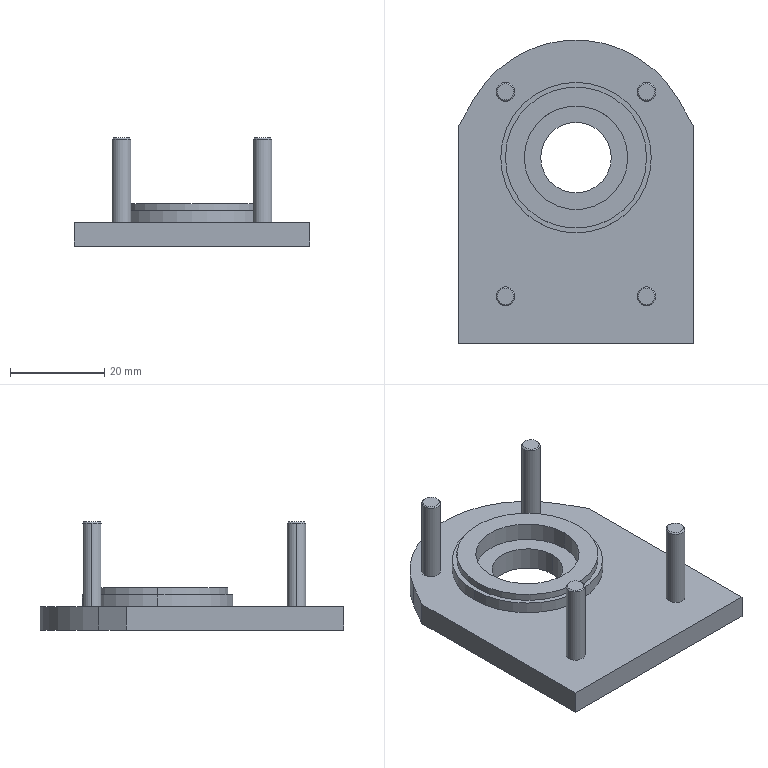Part | SolidWorks | features BaseBody 1 | 1 solid | 39 faces | box 50 x 64.5 x 23 mm | volume 16392 mm3 | cylinder 17 | plane 14 | cone 8 | commonest cylinder face diameters 4 x8 15 x2 22 x2 30 x2 32 x2 50 x1
STEP:
#1=CARTESIAN_POINT('',(-16.75,10.,23.));
#2=VERTEX_POINT('',#1);
#3=CARTESIAN_POINT('',(-13.25,10.,23.));
#4=VERTEX_POINT('',#3);
#5=CARTESIAN_POINT('',(-15.,10.,23.));
#6=DIRECTION('',(0.,0.,-1.));
#7=DIRECTION('',(-1.,0.,0.));
#8=AXIS2_PLACEMENT_3D('',#5,#6,#7);
#9=CIRCLE('',#8,1.75);
#10=EDGE_CURVE('',#2,#4,#9,.T.);
#11=ORIENTED_EDGE('',*,*,#10,.T.);
#12=CARTESIAN_POINT('',(-13.,10.,22.75));
#13=VERTEX_POINT('',#12);
#14=CARTESIAN_POINT('',(-13.125,10.,22.875));
#15=DIRECTION('',(0.7071,0.,-0.7071));
#16=VECTOR('',#15,1000.);
#17=LINE('',#14,#16);
#18=EDGE_CURVE('',#4,#13,#17,.T.);
#19=ORIENTED_EDGE('',*,*,#18,.T.);
#20=CARTESIAN_POINT('',(-17.,10.,22.75));
#21=VERTEX_POINT('',#20);
#22=CARTESIAN_POINT('',(-15.,10.,22.75));
#23=DIRECTION('',(0.,0.,1.));
#24=DIRECTION('',(-1.,0.,0.));
#25=AXIS2_PLACEMENT_3D('',#22,#23,#24);
#26=CIRCLE('',#25,2.);
#27=EDGE_CURVE('',#13,#21,#26,.T.);
#28=ORIENTED_EDGE('',*,*,#27,.T.);
#29=CARTESIAN_POINT('',(-16.875,10.,22.875));
#30=DIRECTION('',(-0.7071,0.,-0.7071));
#31=VECTOR('',#30,1000.);
#32=LINE('',#29,#31);
#33=EDGE_CURVE('',#2,#21,#32,.T.);
#34=ORIENTED_EDGE('',*,*,#33,.F.);
#35=EDGE_LOOP('',(#11,#19,#28,#34));
#36=FACE_OUTER_BOUND('',#35,.T.);
#37=CARTESIAN_POINT('',(-15.,10.,22.875));
#38=DIRECTION('',(0.,0.,-1.));
#39=DIRECTION('',(-1.,0.,0.));
#40=AXIS2_PLACEMENT_3D('',#37,#38,#39);
#41=CONICAL_SURFACE('',#40,1.875,0.7854);
#42=ADVANCED_FACE('',(#36),#41,.T.);
#43=ORIENTED_EDGE('',*,*,#27,.F.);
#44=CARTESIAN_POINT('',(-13.,10.,5.));
#45=VERTEX_POINT('',#44);
#46=CARTESIAN_POINT('',(-13.,10.,5.));
#47=DIRECTION('',(0.,0.,-1.));
#48=VECTOR('',#47,1000.);
#49=LINE('',#46,#48);
#50=EDGE_CURVE('',#13,#45,#49,.T.);
#51=ORIENTED_EDGE('',*,*,#50,.T.);
#52=CARTESIAN_POINT('',(-17.,10.,5.));
#53=VERTEX_POINT('',#52);
#54=CARTESIAN_POINT('',(-15.,10.,5.));
#55=DIRECTION('',(0.,0.,-1.));
#56=DIRECTION('',(-1.,0.,0.));
#57=AXIS2_PLACEMENT_3D('',#54,#55,#56);
#58=CIRCLE('',#57,2.);
#59=EDGE_CURVE('',#53,#45,#58,.T.);
#60=ORIENTED_EDGE('',*,*,#59,.F.);
#61=CARTESIAN_POINT('',(-17.,10.,5.));
#62=DIRECTION('',(0.,0.,-1.));
#63=VECTOR('',#62,1000.);
#64=LINE('',#61,#63);
#65=EDGE_CURVE('',#21,#53,#64,.T.);
#66=ORIENTED_EDGE('',*,*,#65,.F.);
#67=EDGE_LOOP('',(#43,#51,#60,#66));
#68=FACE_OUTER_BOUND('',#67,.T.);
#69=CARTESIAN_POINT('',(-15.,10.,5.));
#70=DIRECTION('',(0.,0.,-1.));
#71=DIRECTION('',(-1.,0.,0.));
#72=AXIS2_PLACEMENT_3D('',#69,#70,#71);
#73=CYLINDRICAL_SURFACE('',#72,2.);
#74=ADVANCED_FACE('',(#68),#73,.T.);
#75=CARTESIAN_POINT('',(13.25,10.,23.));
#76=VERTEX_POINT('',#75);
#77=CARTESIAN_POINT('',(16.75,10.,23.));
#78=VERTEX_POINT('',#77);
#79=CARTESIAN_POINT('',(15.,10.,23.));
#80=DIRECTION('',(0.,0.,-1.));
#81=DIRECTION('',(-1.,0.,0.));
#82=AXIS2_PLACEMENT_3D('',#79,#80,#81);
#83=CIRCLE('',#82,1.75);
#84=EDGE_CURVE('',#76,#78,#83,.T.);
#85=ORIENTED_EDGE('',*,*,#84,.T.);
#86=CARTESIAN_POINT('',(17.,10.,22.75));
#87=VERTEX_POINT('',#86);
#88=CARTESIAN_POINT('',(16.875,10.,22.875));
#89=DIRECTION('',(0.7071,0.,-0.7071));
#90=VECTOR('',#89,1000.);
#91=LINE('',#88,#90);
#92=EDGE_CURVE('',#78,#87,#91,.T.);
#93=ORIENTED_EDGE('',*,*,#92,.T.);
#94=CARTESIAN_POINT('',(13.,10.,22.75));
#95=VERTEX_POINT('',#94);
#96=CARTESIAN_POINT('',(15.,10.,22.75));
#97=DIRECTION('',(0.,0.,1.));
#98=DIRECTION('',(-1.,0.,0.));
#99=AXIS2_PLACEMENT_3D('',#96,#97,#98);
#100=CIRCLE('',#99,2.);
#101=EDGE_CURVE('',#87,#95,#100,.T.);
#102=ORIENTED_EDGE('',*,*,#101,.T.);
#103=CARTESIAN_POINT('',(13.125,10.,22.875));
#104=DIRECTION('',(-0.7071,0.,-0.7071));
#105=VECTOR('',#104,1000.);
#106=LINE('',#103,#105);
#107=EDGE_CURVE('',#76,#95,#106,.T.);
#108=ORIENTED_EDGE('',*,*,#107,.F.);
#109=EDGE_LOOP('',(#85,#93,#102,#108));
#110=FACE_OUTER_BOUND('',#109,.T.);
#111=CARTESIAN_POINT('',(15.,10.,22.875));
#112=DIRECTION('',(0.,0.,-1.));
#113=DIRECTION('',(-1.,0.,0.));
#114=AXIS2_PLACEMENT_3D('',#111,#112,#113);
#115=CONICAL_SURFACE('',#114,1.875,0.7854);
#116=ADVANCED_FACE('',(#110),#115,.T.);
#117=ORIENTED_EDGE('',*,*,#101,.F.);
#118=CARTESIAN_POINT('',(17.,10.,5.));
#119=VERTEX_POINT('',#118);
#120=CARTESIAN_POINT('',(17.,10.,5.));
#121=DIRECTION('',(0.,0.,-1.));
#122=VECTOR('',#121,1000.);
#123=LINE('',#120,#122);
#124=EDGE_CURVE('',#87,#119,#123,.T.);
#125=ORIENTED_EDGE('',*,*,#124,.T.);
#126=CARTESIAN_POINT('',(13.,10.,5.));
#127=VERTEX_POINT('',#126);
#128=CARTESIAN_POINT('',(15.,10.,5.));
#129=DIRECTION('',(0.,0.,-1.));
#130=DIRECTION('',(-1.,0.,0.));
#131=AXIS2_PLACEMENT_3D('',#128,#129,#130);
#132=CIRCLE('',#131,2.);
#133=EDGE_CURVE('',#127,#119,#132,.T.);
#134=ORIENTED_EDGE('',*,*,#133,.F.);
#135=CARTESIAN_POINT('',(13.,10.,5.));
#136=DIRECTION('',(0.,0.,-1.));
#137=VECTOR('',#136,1000.);
#138=LINE('',#135,#137);
#139=EDGE_CURVE('',#95,#127,#138,.T.);
#140=ORIENTED_EDGE('',*,*,#139,.F.);
#141=EDGE_LOOP('',(#117,#125,#134,#140));
#142=FACE_OUTER_BOUND('',#141,.T.);
#143=CARTESIAN_POINT('',(15.,10.,5.));
#144=DIRECTION('',(0.,0.,-1.));
#145=DIRECTION('',(-1.,0.,0.));
#146=AXIS2_PLACEMENT_3D('',#143,#144,#145);
#147=CYLINDRICAL_SURFACE('',#146,2.);
#148=ADVANCED_FACE('',(#142),#147,.T.);
#149=CARTESIAN_POINT('',(13.25,53.473,23.));
#150=VERTEX_POINT('',#149);
#151=CARTESIAN_POINT('',(16.75,53.473,23.));
#152=VERTEX_POINT('',#151);
#153=CARTESIAN_POINT('',(15.,53.473,23.));
#154=DIRECTION('',(0.,0.,-1.));
#155=DIRECTION('',(-1.,0.,0.));
#156=AXIS2_PLACEMENT_3D('',#153,#154,#155);
#157=CIRCLE('',#156,1.75);
#158=EDGE_CURVE('',#150,#152,#157,.T.);
#159=ORIENTED_EDGE('',*,*,#158,.T.);
#160=CARTESIAN_POINT('',(17.,53.473,22.75));
#161=VERTEX_POINT('',#160);
#162=CARTESIAN_POINT('',(16.875,53.473,22.875));
#163=DIRECTION('',(0.7071,0.,-0.7071));
#164=VECTOR('',#163,1000.);
#165=LINE('',#162,#164);
#166=EDGE_CURVE('',#152,#161,#165,.T.);
#167=ORIENTED_EDGE('',*,*,#166,.T.);
#168=CARTESIAN_POINT('',(13.,53.473,22.75));
#169=VERTEX_POINT('',#168);
#170=CARTESIAN_POINT('',(15.,53.473,22.75));
#171=DIRECTION('',(0.,0.,1.));
#172=DIRECTION('',(-1.,0.,0.));
#173=AXIS2_PLACEMENT_3D('',#170,#171,#172);
#174=CIRCLE('',#173,2.);
#175=EDGE_CURVE('',#161,#169,#174,.T.);
#176=ORIENTED_EDGE('',*,*,#175,.T.);
#177=CARTESIAN_POINT('',(13.125,53.473,22.875));
#178=DIRECTION('',(-0.7071,0.,-0.7071));
#179=VECTOR('',#178,1000.);
#180=LINE('',#177,#179);
#181=EDGE_CURVE('',#150,#169,#180,.T.);
#182=ORIENTED_EDGE('',*,*,#181,.F.);
#183=EDGE_LOOP('',(#159,#167,#176,#182));
#184=FACE_OUTER_BOUND('',#183,.T.);
#185=CARTESIAN_POINT('',(15.,53.473,22.875));
#186=DIRECTION('',(0.,0.,-1.));
#187=DIRECTION('',(-1.,0.,0.));
#188=AXIS2_PLACEMENT_3D('',#185,#186,#187);
#189=CONICAL_SURFACE('',#188,1.875,0.7854);
#190=ADVANCED_FACE('',(#184),#189,.T.);
#191=ORIENTED_EDGE('',*,*,#175,.F.);
#192=CARTESIAN_POINT('',(17.,53.473,5.));
#193=VERTEX_POINT('',#192);
#194=CARTESIAN_POINT('',(17.,53.473,5.));
#195=DIRECTION('',(0.,0.,-1.));
#196=VECTOR('',#195,1000.);
#197=LINE('',#194,#196);
#198=EDGE_CURVE('',#161,#193,#197,.T.);
#199=ORIENTED_EDGE('',*,*,#198,.T.);
#200=CARTESIAN_POINT('',(13.,53.473,5.));
#201=VERTEX_POINT('',#200);
#202=CARTESIAN_POINT('',(15.,53.473,5.));
#203=DIRECTION('',(0.,0.,-1.));
#204=DIRECTION('',(-1.,0.,0.));
#205=AXIS2_PLACEMENT_3D('',#202,#203,#204);
#206=CIRCLE('',#205,2.);
#207=EDGE_CURVE('',#201,#193,#206,.T.);
#208=ORIENTED_EDGE('',*,*,#207,.F.);
#209=CARTESIAN_POINT('',(13.,53.473,5.));
#210=DIRECTION('',(0.,0.,-1.));
#211=VECTOR('',#210,1000.);
#212=LINE('',#209,#211);
#213=EDGE_CURVE('',#169,#201,#212,.T.);
#214=ORIENTED_EDGE('',*,*,#213,.F.);
#215=EDGE_LOOP('',(#191,#199,#208,#214));
#216=FACE_OUTER_BOUND('',#215,.T.);
#217=CARTESIAN_POINT('',(15.,53.473,5.));
#218=DIRECTION('',(0.,0.,-1.));
#219=DIRECTION('',(-1.,0.,0.));
#220=AXIS2_PLACEMENT_3D('',#217,#218,#219);
#221=CYLINDRICAL_SURFACE('',#220,2.);
#222=ADVANCED_FACE('',(#216),#221,.T.);
#223=CARTESIAN_POINT('',(-16.75,53.473,23.));
#224=VERTEX_POINT('',#223);
#225=CARTESIAN_POINT('',(-13.25,53.473,23.));
#226=VERTEX_POINT('',#225);
#227=CARTESIAN_POINT('',(-15.,53.473,23.));
#228=DIRECTION('',(0.,0.,-1.));
#229=DIRECTION('',(-1.,0.,0.));
#230=AXIS2_PLACEMENT_3D('',#227,#228,#229);
#231=CIRCLE('',#230,1.75);
#232=EDGE_CURVE('',#224,#226,#231,.T.);
#233=ORIENTED_EDGE('',*,*,#232,.T.);
#234=CARTESIAN_POINT('',(-13.,53.473,22.75));
#235=VERTEX_POINT('',#234);
#236=CARTESIAN_POINT('',(-13.125,53.473,22.875));
#237=DIRECTION('',(0.7071,0.,-0.7071));
#238=VECTOR('',#237,1000.);
#239=LINE('',#236,#238);
#240=EDGE_CURVE('',#226,#235,#239,.T.);
#241=ORIENTED_EDGE('',*,*,#240,.T.);
#242=CARTESIAN_POINT('',(-17.,53.473,22.75));
#243=VERTEX_POINT('',#242);
#244=CARTESIAN_POINT('',(-15.,53.473,22.75));
#245=DIRECTION('',(0.,0.,1.));
#246=DIRECTION('',(-1.,0.,0.));
#247=AXIS2_PLACEMENT_3D('',#244,#245,#246);
#248=CIRCLE('',#247,2.);
#249=EDGE_CURVE('',#235,#243,#248,.T.);
#250=ORIENTED_EDGE('',*,*,#249,.T.);
#251=CARTESIAN_POINT('',(-16.875,53.473,22.875));
#252=DIRECTION('',(-0.7071,0.,-0.7071));
#253=VECTOR('',#252,1000.);
#254=LINE('',#251,#253);
#255=EDGE_CURVE('',#224,#243,#254,.T.);
#256=ORIENTED_EDGE('',*,*,#255,.F.);
#257=EDGE_LOOP('',(#233,#241,#250,#256));
#258=FACE_OUTER_BOUND('',#257,.T.);
#259=CARTESIAN_POINT('',(-15.,53.473,22.875));
#260=DIRECTION('',(0.,0.,-1.));
#261=DIRECTION('',(-1.,0.,0.));
#262=AXIS2_PLACEMENT_3D('',#259,#260,#261);
#263=CONICAL_SURFACE('',#262,1.875,0.7854);
#264=ADVANCED_FACE('',(#258),#263,.T.);
#265=ORIENTED_EDGE('',*,*,#249,.F.);
#266=CARTESIAN_POINT('',(-13.,53.473,5.));
#267=VERTEX_POINT('',#266);
#268=CARTESIAN_POINT('',(-13.,53.473,5.));
#269=DIRECTION('',(0.,0.,-1.));
#270=VECTOR('',#269,1000.);
#271=LINE('',#268,#270);
#272=EDGE_CURVE('',#235,#267,#271,.T.);
#273=ORIENTED_EDGE('',*,*,#272,.T.);
#274=CARTESIAN_POINT('',(-17.,53.473,5.));
#275=VERTEX_POINT('',#274);
#276=CARTESIAN_POINT('',(-15.,53.473,5.));
#277=DIRECTION('',(0.,0.,-1.));
#278=DIRECTION('',(-1.,0.,0.));
#279=AXIS2_PLACEMENT_3D('',#276,#277,#278);
#280=CIRCLE('',#279,2.);
#281=EDGE_CURVE('',#275,#267,#280,.T.);
#282=ORIENTED_EDGE('',*,*,#281,.F.);
#283=CARTESIAN_POINT('',(-17.,53.473,5.));
#284=DIRECTION('',(0.,0.,-1.));
#285=VECTOR('',#284,1000.);
#286=LINE('',#283,#285);
#287=EDGE_CURVE('',#243,#275,#286,.T.);
#288=ORIENTED_EDGE('',*,*,#287,.F.);
#289=EDGE_LOOP('',(#265,#273,#282,#288));
#290=FACE_OUTER_BOUND('',#289,.T.);
#291=CARTESIAN_POINT('',(-15.,53.473,5.));
#292=DIRECTION('',(0.,0.,-1.));
#293=DIRECTION('',(-1.,0.,0.));
#294=AXIS2_PLACEMENT_3D('',#291,#292,#293);
#295=CYLINDRICAL_SURFACE('',#294,2.);
#296=ADVANCED_FACE('',(#290),#295,.T.);
#297=CARTESIAN_POINT('',(7.5,39.5,0.));
#298=VERTEX_POINT('',#297);
#299=CARTESIAN_POINT('',(-7.5,39.5,0.));
#300=VERTEX_POINT('',#299);
#301=CARTESIAN_POINT('',(0.,39.5,0.));
#302=DIRECTION('',(0.,0.,1.));
#303=DIRECTION('',(-1.,0.,0.));
#304=AXIS2_PLACEMENT_3D('',#301,#302,#303);
#305=CIRCLE('',#304,7.5);
#306=EDGE_CURVE('',#298,#300,#305,.T.);
#307=ORIENTED_EDGE('',*,*,#306,.F.);
#308=CARTESIAN_POINT('',(7.5,39.5,5.));
#309=VERTEX_POINT('',#308);
#310=CARTESIAN_POINT('',(7.5,39.5,5.));
#311=DIRECTION('',(0.,0.,1.));
#312=VECTOR('',#311,1000.);
#313=LINE('',#310,#312);
#314=EDGE_CURVE('',#298,#309,#313,.T.);
#315=ORIENTED_EDGE('',*,*,#314,.T.);
#316=CARTESIAN_POINT('',(-7.5,39.5,5.));
#317=VERTEX_POINT('',#316);
#318=CARTESIAN_POINT('',(0.,39.5,5.));
#319=DIRECTION('',(0.,0.,-1.));
#320=DIRECTION('',(-1.,0.,0.));
#321=AXIS2_PLACEMENT_3D('',#318,#319,#320);
#322=CIRCLE('',#321,7.5);
#323=EDGE_CURVE('',#317,#309,#322,.T.);
#324=ORIENTED_EDGE('',*,*,#323,.F.);
#325=CARTESIAN_POINT('',(-7.5,39.5,5.));
#326=DIRECTION('',(0.,0.,1.));
#327=VECTOR('',#326,1000.);
#328=LINE('',#325,#327);
#329=EDGE_CURVE('',#300,#317,#328,.T.);
#330=ORIENTED_EDGE('',*,*,#329,.F.);
#331=EDGE_LOOP('',(#307,#315,#324,#330));
#332=FACE_OUTER_BOUND('',#331,.T.);
#333=CARTESIAN_POINT('',(0.,39.5,5.));
#334=DIRECTION('',(0.,0.,1.));
#335=DIRECTION('',(-1.,0.,0.));
#336=AXIS2_PLACEMENT_3D('',#333,#334,#335);
#337=CYLINDRICAL_SURFACE('',#336,7.5);
#338=ADVANCED_FACE('',(#332),#337,.F.);
#339=CARTESIAN_POINT('',(-15.,39.5,7.5));
#340=VERTEX_POINT('',#339);
#341=CARTESIAN_POINT('',(15.,39.5,7.5));
#342=VERTEX_POINT('',#341);
#343=CARTESIAN_POINT('',(0.,39.5,7.5));
#344=DIRECTION('',(0.,0.,1.));
#345=DIRECTION('',(-1.,0.,0.));
#346=AXIS2_PLACEMENT_3D('',#343,#344,#345);
#347=CIRCLE('',#346,15.);
#348=EDGE_CURVE('',#340,#342,#347,.T.);
#349=ORIENTED_EDGE('',*,*,#348,.T.);
#350=CARTESIAN_POINT('',(15.,39.5,9.));
#351=VERTEX_POINT('',#350);
#352=CARTESIAN_POINT('',(15.,39.5,9.));
#353=DIRECTION('',(0.,0.,1.));
#354=VECTOR('',#353,1000.);
#355=LINE('',#352,#354);
#356=EDGE_CURVE('',#342,#351,#355,.T.);
#357=ORIENTED_EDGE('',*,*,#356,.T.);
#358=CARTESIAN_POINT('',(-15.,39.5,9.));
#359=VERTEX_POINT('',#358);
#360=CARTESIAN_POINT('',(0.,39.5,9.));
#361=DIRECTION('',(0.,0.,1.));
#362=DIRECTION('',(-1.,0.,0.));
#363=AXIS2_PLACEMENT_3D('',#360,#361,#362);
#364=CIRCLE('',#363,15.);
#365=EDGE_CURVE('',#359,#351,#364,.T.);
#366=ORIENTED_EDGE('',*,*,#365,.F.);
#367=CARTESIAN_POINT('',(-15.,39.5,9.));
#368=DIRECTION('',(0.,0.,1.));
#369=VECTOR('',#368,1000.);
#370=LINE('',#367,#369);
#371=EDGE_CURVE('',#340,#359,#370,.T.);
#372=ORIENTED_EDGE('',*,*,#371,.F.);
#373=EDGE_LOOP('',(#349,#357,#366,#372));
#374=FACE_OUTER_BOUND('',#373,.T.);
#375=CARTESIAN_POINT('',(0.,39.5,9.));
#376=DIRECTION('',(0.,0.,1.));
#377=DIRECTION('',(-1.,0.,0.));
#378=AXIS2_PLACEMENT_3D('',#375,#376,#377);
#379=CYLINDRICAL_SURFACE('',#378,15.);
#380=ADVANCED_FACE('',(#374),#379,.T.);
#381=CARTESIAN_POINT('',(11.,39.5,9.));
#382=VERTEX_POINT('',#381);
#383=CARTESIAN_POINT('',(-11.,39.5,9.));
#384=VERTEX_POINT('',#383);
#385=CARTESIAN_POINT('',(0.,39.5,9.));
#386=DIRECTION('',(0.,0.,-1.));
#387=DIRECTION('',(-1.,0.,0.));
#388=AXIS2_PLACEMENT_3D('',#385,#386,#387);
#389=CIRCLE('',#388,11.);
#390=EDGE_CURVE('',#382,#384,#389,.T.);
#391=ORIENTED_EDGE('',*,*,#390,.F.);
#392=CARTESIAN_POINT('',(11.,39.5,5.));
#393=VERTEX_POINT('',#392);
#394=CARTESIAN_POINT('',(11.,39.5,5.));
#395=DIRECTION('',(0.,0.,-1.));
#396=VECTOR('',#395,1000.);
#397=LINE('',#394,#396);
#398=EDGE_CURVE('',#382,#393,#397,.T.);
#399=ORIENTED_EDGE('',*,*,#398,.T.);
#400=CARTESIAN_POINT('',(-11.,39.5,5.));
#401=VERTEX_POINT('',#400);
#402=CARTESIAN_POINT('',(0.,39.5,5.));
#403=DIRECTION('',(0.,0.,1.));
#404=DIRECTION('',(-1.,0.,0.));
#405=AXIS2_PLACEMENT_3D('',#402,#403,#404);
#406=CIRCLE('',#405,11.);
#407=EDGE_CURVE('',#401,#393,#406,.T.);
#408=ORIENTED_EDGE('',*,*,#407,.F.);
#409=CARTESIAN_POINT('',(-11.,39.5,5.));
#410=DIRECTION('',(0.,0.,-1.));
#411=VECTOR('',#410,1000.);
#412=LINE('',#409,#411);
#413=EDGE_CURVE('',#384,#401,#412,.T.);
#414=ORIENTED_EDGE('',*,*,#413,.F.);
#415=EDGE_LOOP('',(#391,#399,#408,#414));
#416=FACE_OUTER_BOUND('',#415,.T.);
#417=CARTESIAN_POINT('',(0.,39.5,5.));
#418=DIRECTION('',(0.,0.,-1.));
#419=DIRECTION('',(-1.,0.,0.));
#420=AXIS2_PLACEMENT_3D('',#417,#418,#419);
#421=CYLINDRICAL_SURFACE('',#420,11.);
#422=ADVANCED_FACE('',(#416),#421,.F.);
#423=CARTESIAN_POINT('',(-16.,39.5,7.5));
#424=VERTEX_POINT('',#423);
#425=CARTESIAN_POINT('',(16.,39.5,7.5));
#426=VERTEX_POINT('',#425);
#427=CARTESIAN_POINT('',(0.,39.5,7.5));
#428=DIRECTION('',(0.,0.,-1.));
#429=DIRECTION('',(-1.,0.,0.));
#430=AXIS2_PLACEMENT_3D('',#427,#428,#429);
#431=CIRCLE('',#430,16.);
#432=EDGE_CURVE('',#424,#426,#431,.T.);
#433=ORIENTED_EDGE('',*,*,#432,.T.);
#434=CARTESIAN_POINT('',(16.,39.5,5.));
#435=VERTEX_POINT('',#434);
#436=CARTESIAN_POINT('',(16.,39.5,5.));
#437=DIRECTION('',(0.,0.,-1.));
#438=VECTOR('',#437,1000.);
#439=LINE('',#436,#438);
#440=EDGE_CURVE('',#426,#435,#439,.T.);
#441=ORIENTED_EDGE('',*,*,#440,.T.);
#442=CARTESIAN_POINT('',(-16.,39.5,5.));
#443=VERTEX_POINT('',#442);
#444=CARTESIAN_POINT('',(0.,39.5,5.));
#445=DIRECTION('',(0.,0.,-1.));
#446=DIRECTION('',(-1.,0.,0.));
#447=AXIS2_PLACEMENT_3D('',#444,#445,#446);
#448=CIRCLE('',#447,16.);
#449=EDGE_CURVE('',#443,#435,#448,.T.);
#450=ORIENTED_EDGE('',*,*,#449,.F.);
#451=CARTESIAN_POINT('',(-16.,39.5,5.));
#452=DIRECTION('',(0.,0.,-1.));
#453=VECTOR('',#452,1000.);
#454=LINE('',#451,#453);
#455=EDGE_CURVE('',#424,#443,#454,.T.);
#456=ORIENTED_EDGE('',*,*,#455,.F.);
#457=EDGE_LOOP('',(#433,#441,#450,#456));
#458=FACE_OUTER_BOUND('',#457,.T.);
#459=CARTESIAN_POINT('',(0.,39.5,5.));
#460=DIRECTION('',(0.,0.,-1.));
#461=DIRECTION('',(-1.,0.,0.));
#462=AXIS2_PLACEMENT_3D('',#459,#460,#461);
#463=CYLINDRICAL_SURFACE('',#462,16.);
#464=ADVANCED_FACE('',(#458),#463,.T.);
#465=ORIENTED_EDGE('',*,*,#10,.F.);
#466=CARTESIAN_POINT('',(-15.,10.,23.));
#467=DIRECTION('',(0.,0.,-1.));
#468=DIRECTION('',(-1.,0.,0.));
#469=AXIS2_PLACEMENT_3D('',#466,#467,#468);
#470=CIRCLE('',#469,1.75);
#471=EDGE_CURVE('',#4,#2,#470,.T.);
#472=ORIENTED_EDGE('',*,*,#471,.F.);
#473=EDGE_LOOP('',(#465,#472));
#474=FACE_OUTER_BOUND('',#473,.T.);
#475=CARTESIAN_POINT('',(-15.,10.,23.));
#476=DIRECTION('',(0.,0.,1.));
#477=DIRECTION('',(1.,0.,0.));
#478=AXIS2_PLACEMENT_3D('',#475,#476,#477);
#479=PLANE('',#478);
#480=ADVANCED_FACE('',(#474),#479,.T.);
#481=ORIENTED_EDGE('',*,*,#84,.F.);
#482=CARTESIAN_POINT('',(15.,10.,23.));
#483=DIRECTION('',(0.,0.,-1.));
#484=DIRECTION('',(-1.,0.,0.));
#485=AXIS2_PLACEMENT_3D('',#482,#483,#484);
#486=CIRCLE('',#485,1.75);
#487=EDGE_CURVE('',#78,#76,#486,.T.);
#488=ORIENTED_EDGE('',*,*,#487,.F.);
#489=EDGE_LOOP('',(#481,#488));
#490=FACE_OUTER_BOUND('',#489,.T.);
#491=CARTESIAN_POINT('',(15.,10.,23.));
#492=DIRECTION('',(0.,0.,1.));
#493=DIRECTION('',(1.,0.,0.));
#494=AXIS2_PLACEMENT_3D('',#491,#492,#493);
#495=PLANE('',#494);
#496=ADVANCED_FACE('',(#490),#495,.T.);
#497=ORIENTED_EDGE('',*,*,#158,.F.);
#498=CARTESIAN_POINT('',(15.,53.473,23.));
#499=DIRECTION('',(0.,0.,-1.));
#500=DIRECTION('',(-1.,0.,0.));
#501=AXIS2_PLACEMENT_3D('',#498,#499,#500);
#502=CIRCLE('',#501,1.75);
#503=EDGE_CURVE('',#152,#150,#502,.T.);
#504=ORIENTED_EDGE('',*,*,#503,.F.);
#505=EDGE_LOOP('',(#497,#504));
#506=FACE_OUTER_BOUND('',#505,.T.);
#507=CARTESIAN_POINT('',(15.,53.473,23.));
#508=DIRECTION('',(0.,0.,1.));
#509=DIRECTION('',(1.,0.,0.));
#510=AXIS2_PLACEMENT_3D('',#507,#508,#509);
#511=PLANE('',#510);
#512=ADVANCED_FACE('',(#506),#511,.T.);
#513=ORIENTED_EDGE('',*,*,#232,.F.);
#514=CARTESIAN_POINT('',(-15.,53.473,23.));
#515=DIRECTION('',(0.,0.,-1.));
#516=DIRECTION('',(-1.,0.,0.));
#517=AXIS2_PLACEMENT_3D('',#514,#515,#516);
#518=CIRCLE('',#517,1.75);
#519=EDGE_CURVE('',#226,#224,#518,.T.);
#520=ORIENTED_EDGE('',*,*,#519,.F.);
#521=EDGE_LOOP('',(#513,#520));
#522=FACE_OUTER_BOUND('',#521,.T.);
#523=CARTESIAN_POINT('',(-15.,53.473,23.));
#524=DIRECTION('',(0.,0.,1.));
#525=DIRECTION('',(1.,0.,0.));
#526=AXIS2_PLACEMENT_3D('',#523,#524,#525);
#527=PLANE('',#526);
#528=ADVANCED_FACE('',(#522),#527,.T.);
#529=ORIENTED_EDGE('',*,*,#348,.F.);
#530=CARTESIAN_POINT('',(0.,39.5,7.5));
#531=DIRECTION('',(0.,0.,1.));
#532=DIRECTION('',(-1.,0.,0.));
#533=AXIS2_PLACEMENT_3D('',#530,#531,#532);
#534=CIRCLE('',#533,15.);
#535=EDGE_CURVE('',#342,#340,#534,.T.);
#536=ORIENTED_EDGE('',*,*,#535,.F.);
#537=EDGE_LOOP('',(#529,#536));
#538=FACE_BOUND('',#537,.T.);
#539=ORIENTED_EDGE('',*,*,#432,.F.);
#540=CARTESIAN_POINT('',(0.,39.5,7.5));
#541=DIRECTION('',(0.,0.,-1.));
#542=DIRECTION('',(-1.,0.,0.));
#543=AXIS2_PLACEMENT_3D('',#540,#541,#542);
#544=CIRCLE('',#543,16.);
#545=EDGE_CURVE('',#426,#424,#544,.T.);
#546=ORIENTED_EDGE('',*,*,#545,.F.);
#547=EDGE_LOOP('',(#539,#546));
#548=FACE_OUTER_BOUND('',#547,.T.);
#549=CARTESIAN_POINT('',(0.,39.5,7.5));
#550=DIRECTION('',(0.,0.,1.));
#551=DIRECTION('',(1.,0.,0.));
#552=AXIS2_PLACEMENT_3D('',#549,#550,#551);
#553=PLANE('',#552);
#554=ADVANCED_FACE('',(#538,#548),#553,.T.);
#555=CARTESIAN_POINT('',(0.,39.5,9.));
#556=DIRECTION('',(0.,0.,-1.));
#557=DIRECTION('',(-1.,0.,0.));
#558=AXIS2_PLACEMENT_3D('',#555,#556,#557);
#559=CIRCLE('',#558,11.);
#560=EDGE_CURVE('',#384,#382,#559,.T.);
#561=ORIENTED_EDGE('',*,*,#560,.T.);
#562=ORIENTED_EDGE('',*,*,#390,.T.);
#563=EDGE_LOOP('',(#561,#562));
#564=FACE_BOUND('',#563,.T.);
#565=ORIENTED_EDGE('',*,*,#365,.T.);
#566=CARTESIAN_POINT('',(0.,39.5,9.));
#567=DIRECTION('',(0.,0.,1.));
#568=DIRECTION('',(-1.,0.,0.));
#569=AXIS2_PLACEMENT_3D('',#566,#567,#568);
#570=CIRCLE('',#569,15.);
#571=EDGE_CURVE('',#351,#359,#570,.T.);
#572=ORIENTED_EDGE('',*,*,#571,.T.);
#573=EDGE_LOOP('',(#565,#572));
#574=FACE_OUTER_BOUND('',#573,.T.);
#575=CARTESIAN_POINT('',(0.,39.5,9.));
#576=DIRECTION('',(0.,0.,1.));
#577=DIRECTION('',(1.,0.,0.));
#578=AXIS2_PLACEMENT_3D('',#575,#576,#577);
#579=PLANE('',#578);
#580=ADVANCED_FACE('',(#564,#574),#579,.T.);
#581=ORIENTED_EDGE('',*,*,#207,.T.);
#582=CARTESIAN_POINT('',(15.,53.473,5.));
#583=DIRECTION('',(0.,0.,-1.));
#584=DIRECTION('',(-1.,0.,0.));
#585=AXIS2_PLACEMENT_3D('',#582,#583,#584);
#586=CIRCLE('',#585,2.);
#587=EDGE_CURVE('',#193,#201,#586,.T.);
#588=ORIENTED_EDGE('',*,*,#587,.T.);
#589=EDGE_LOOP('',(#581,#588));
#590=FACE_BOUND('',#589,.T.);
#591=ORIENTED_EDGE('',*,*,#133,.T.);
#592=CARTESIAN_POINT('',(15.,10.,5.));
#593=DIRECTION('',(0.,0.,-1.));
#594=DIRECTION('',(-1.,0.,0.));
#595=AXIS2_PLACEMENT_3D('',#592,#593,#594);
#596=CIRCLE('',#595,2.);
#597=EDGE_CURVE('',#119,#127,#596,.T.);
#598=ORIENTED_EDGE('',*,*,#597,.T.);
#599=EDGE_LOOP('',(#591,#598));
#600=FACE_BOUND('',#599,.T.);
#601=ORIENTED_EDGE('',*,*,#59,.T.);
#602=CARTESIAN_POINT('',(-15.,10.,5.));
#603=DIRECTION('',(0.,0.,-1.));
#604=DIRECTION('',(-1.,0.,0.));
#605=AXIS2_PLACEMENT_3D('',#602,#603,#604);
#606=CIRCLE('',#605,2.);
#607=EDGE_CURVE('',#45,#53,#606,.T.);
#608=ORIENTED_EDGE('',*,*,#607,.T.);
#609=EDGE_LOOP('',(#601,#608));
#610=FACE_BOUND('',#609,.T.);
#611=ORIENTED_EDGE('',*,*,#281,.T.);
#612=CARTESIAN_POINT('',(-15.,53.473,5.));
#613=DIRECTION('',(0.,0.,-1.));
#614=DIRECTION('',(-1.,0.,0.));
#615=AXIS2_PLACEMENT_3D('',#612,#613,#614);
#616=CIRCLE('',#615,2.);
#617=EDGE_CURVE('',#267,#275,#616,.T.);
#618=ORIENTED_EDGE('',*,*,#617,.T.);
#619=EDGE_LOOP('',(#611,#618));
#620=FACE_BOUND('',#619,.T.);
#621=ORIENTED_EDGE('',*,*,#449,.T.);
#622=CARTESIAN_POINT('',(0.,39.5,5.));
#623=DIRECTION('',(0.,0.,-1.));
#624=DIRECTION('',(-1.,0.,0.));
#625=AXIS2_PLACEMENT_3D('',#622,#623,#624);
#626=CIRCLE('',#625,16.);
#627=EDGE_CURVE('',#435,#443,#626,.T.);
#628=ORIENTED_EDGE('',*,*,#627,.T.);
#629=EDGE_LOOP('',(#621,#628));
#630=FACE_BOUND('',#629,.T.);
#631=CARTESIAN_POINT('',(-25.,0.,5.));
#632=VERTEX_POINT('',#631);
#633=CARTESIAN_POINT('',(25.,0.,5.));
#634=VERTEX_POINT('',#633);
#635=CARTESIAN_POINT('',(-25.,0.,5.));
#636=DIRECTION('',(1.,0.,0.));
#637=VECTOR('',#636,1000.);
#638=LINE('',#635,#637);
#639=EDGE_CURVE('',#632,#634,#638,.T.);
#640=ORIENTED_EDGE('',*,*,#639,.T.);
#641=CARTESIAN_POINT('',(25.,46.199,5.));
#642=VERTEX_POINT('',#641);
#643=CARTESIAN_POINT('',(25.,0.,5.));
#644=DIRECTION('',(0.,1.,0.));
#645=VECTOR('',#644,1000.);
#646=LINE('',#643,#645);
#647=EDGE_CURVE('',#634,#642,#646,.T.);
#648=ORIENTED_EDGE('',*,*,#647,.T.);
#649=CARTESIAN_POINT('',(21.651,52.,5.));
#650=VERTEX_POINT('',#649);
#651=CARTESIAN_POINT('',(51.673,0.,5.));
#652=DIRECTION('',(-0.5,0.866,0.));
#653=VECTOR('',#652,1000.);
#654=LINE('',#651,#653);
#655=EDGE_CURVE('',#642,#650,#654,.T.);
#656=ORIENTED_EDGE('',*,*,#655,.T.);
#657=CARTESIAN_POINT('',(-21.651,52.,5.));
#658=VERTEX_POINT('',#657);
#659=CARTESIAN_POINT('',(0.,39.5,5.));
#660=DIRECTION('',(0.,0.,1.));
#661=DIRECTION('',(1.,0.,0.));
#662=AXIS2_PLACEMENT_3D('',#659,#660,#661);
#663=CIRCLE('',#662,25.);
#664=EDGE_CURVE('',#650,#658,#663,.T.);
#665=ORIENTED_EDGE('',*,*,#664,.T.);
#666=CARTESIAN_POINT('',(-25.,46.199,5.));
#667=VERTEX_POINT('',#666);
#668=CARTESIAN_POINT('',(-21.651,52.,5.));
#669=DIRECTION('',(-0.5,-0.866,0.));
#670=VECTOR('',#669,1000.);
#671=LINE('',#668,#670);
#672=EDGE_CURVE('',#658,#667,#671,.T.);
#673=ORIENTED_EDGE('',*,*,#672,.T.);
#674=CARTESIAN_POINT('',(-25.,46.199,5.));
#675=DIRECTION('',(0.,-1.,0.));
#676=VECTOR('',#675,1000.);
#677=LINE('',#674,#676);
#678=EDGE_CURVE('',#667,#632,#677,.T.);
#679=ORIENTED_EDGE('',*,*,#678,.T.);
#680=EDGE_LOOP('',(#640,#648,#656,#665,#673,#679));
#681=FACE_OUTER_BOUND('',#680,.T.);
#682=CARTESIAN_POINT('',(0.,26.428,5.));
#683=DIRECTION('',(0.,0.,1.));
#684=DIRECTION('',(1.,0.,0.));
#685=AXIS2_PLACEMENT_3D('',#682,#683,#684);
#686=PLANE('',#685);
#687=ADVANCED_FACE('',(#590,#600,#610,#620,#630,#681),#686,.T.);
#688=CARTESIAN_POINT('',(-25.,46.199,0.));
#689=VERTEX_POINT('',#688);
#690=CARTESIAN_POINT('',(-25.,0.,0.));
#691=VERTEX_POINT('',#690);
#692=CARTESIAN_POINT('',(-25.,46.199,0.));
#693=DIRECTION('',(0.,-1.,0.));
#694=VECTOR('',#693,1000.);
#695=LINE('',#692,#694);
#696=EDGE_CURVE('',#689,#691,#695,.T.);
#697=ORIENTED_EDGE('',*,*,#696,.T.);
#698=CARTESIAN_POINT('',(-25.,0.,0.));
#699=DIRECTION('',(0.,0.,1.));
#700=VECTOR('',#699,1000.);
#701=LINE('',#698,#700);
#702=EDGE_CURVE('',#691,#632,#701,.T.);
#703=ORIENTED_EDGE('',*,*,#702,.T.);
#704=ORIENTED_EDGE('',*,*,#678,.F.);
#705=CARTESIAN_POINT('',(-25.,46.199,0.));
#706=DIRECTION('',(0.,0.,1.));
#707=VECTOR('',#706,1000.);
#708=LINE('',#705,#707);
#709=EDGE_CURVE('',#689,#667,#708,.T.);
#710=ORIENTED_EDGE('',*,*,#709,.F.);
#711=EDGE_LOOP('',(#697,#703,#704,#710));
#712=FACE_OUTER_BOUND('',#711,.T.);
#713=CARTESIAN_POINT('',(-25.,46.199,0.));
#714=DIRECTION('',(-1.,0.,0.));
#715=DIRECTION('',(0.,0.,1.));
#716=AXIS2_PLACEMENT_3D('',#713,#714,#715);
#717=PLANE('',#716);
#718=ADVANCED_FACE('',(#712),#717,.T.);
#719=CARTESIAN_POINT('',(-21.651,52.,0.));
#720=VERTEX_POINT('',#719);
#721=CARTESIAN_POINT('',(-21.651,52.,0.));
#722=DIRECTION('',(-0.5,-0.866,0.));
#723=VECTOR('',#722,1000.);
#724=LINE('',#721,#723);
#725=EDGE_CURVE('',#720,#689,#724,.T.);
#726=ORIENTED_EDGE('',*,*,#725,.T.);
#727=ORIENTED_EDGE('',*,*,#709,.T.);
#728=ORIENTED_EDGE('',*,*,#672,.F.);
#729=CARTESIAN_POINT('',(-21.651,52.,0.));
#730=DIRECTION('',(0.,0.,1.));
#731=VECTOR('',#730,1000.);
#732=LINE('',#729,#731);
#733=EDGE_CURVE('',#720,#658,#732,.T.);
#734=ORIENTED_EDGE('',*,*,#733,.F.);
#735=EDGE_LOOP('',(#726,#727,#728,#734));
#736=FACE_OUTER_BOUND('',#735,.T.);
#737=CARTESIAN_POINT('',(-21.651,52.,0.));
#738=DIRECTION('',(-0.866,0.5,0.));
#739=DIRECTION('',(0.,0.,1.));
#740=AXIS2_PLACEMENT_3D('',#737,#738,#739);
#741=PLANE('',#740);
#742=ADVANCED_FACE('',(#736),#741,.T.);
#743=CARTESIAN_POINT('',(21.651,52.,0.));
#744=VERTEX_POINT('',#743);
#745=CARTESIAN_POINT('',(0.,39.5,0.));
#746=DIRECTION('',(0.,0.,1.));
#747=DIRECTION('',(1.,0.,0.));
#748=AXIS2_PLACEMENT_3D('',#745,#746,#747);
#749=CIRCLE('',#748,25.);
#750=EDGE_CURVE('',#744,#720,#749,.T.);
#751=ORIENTED_EDGE('',*,*,#750,.T.);
#752=ORIENTED_EDGE('',*,*,#733,.T.);
#753=ORIENTED_EDGE('',*,*,#664,.F.);
#754=CARTESIAN_POINT('',(21.651,52.,0.));
#755=DIRECTION('',(0.,0.,1.));
#756=VECTOR('',#755,1000.);
#757=LINE('',#754,#756);
#758=EDGE_CURVE('',#744,#650,#757,.T.);
#759=ORIENTED_EDGE('',*,*,#758,.F.);
#760=EDGE_LOOP('',(#751,#752,#753,#759));
#761=FACE_OUTER_BOUND('',#760,.T.);
#762=CARTESIAN_POINT('',(0.,39.5,0.));
#763=DIRECTION('',(0.,0.,-1.));
#764=DIRECTION('',(1.,0.,0.));
#765=AXIS2_PLACEMENT_3D('',#762,#763,#764);
#766=CYLINDRICAL_SURFACE('',#765,25.);
#767=ADVANCED_FACE('',(#761),#766,.T.);
#768=CARTESIAN_POINT('',(25.,46.199,0.));
#769=VERTEX_POINT('',#768);
#770=CARTESIAN_POINT('',(51.673,0.,0.));
#771=DIRECTION('',(-0.5,0.866,0.));
#772=VECTOR('',#771,1000.);
#773=LINE('',#770,#772);
#774=EDGE_CURVE('',#769,#744,#773,.T.);
#775=ORIENTED_EDGE('',*,*,#774,.T.);
#776=ORIENTED_EDGE('',*,*,#758,.T.);
#777=ORIENTED_EDGE('',*,*,#655,.F.);
#778=CARTESIAN_POINT('',(25.,46.199,0.));
#779=DIRECTION('',(0.,0.,1.));
#780=VECTOR('',#779,1000.);
#781=LINE('',#778,#780);
#782=EDGE_CURVE('',#769,#642,#781,.T.);
#783=ORIENTED_EDGE('',*,*,#782,.F.);
#784=EDGE_LOOP('',(#775,#776,#777,#783));
#785=FACE_OUTER_BOUND('',#784,.T.);
#786=CARTESIAN_POINT('',(25.,46.199,0.));
#787=DIRECTION('',(0.866,0.5,0.));
#788=DIRECTION('',(0.,0.,-1.));
#789=AXIS2_PLACEMENT_3D('',#786,#787,#788);
#790=PLANE('',#789);
#791=ADVANCED_FACE('',(#785),#790,.T.);
#792=CARTESIAN_POINT('',(25.,0.,0.));
#793=VERTEX_POINT('',#792);
#794=CARTESIAN_POINT('',(25.,0.,0.));
#795=DIRECTION('',(0.,1.,0.));
#796=VECTOR('',#795,1000.);
#797=LINE('',#794,#796);
#798=EDGE_CURVE('',#793,#769,#797,.T.);
#799=ORIENTED_EDGE('',*,*,#798,.T.);
#800=ORIENTED_EDGE('',*,*,#782,.T.);
#801=ORIENTED_EDGE('',*,*,#647,.F.);
#802=CARTESIAN_POINT('',(25.,0.,0.));
#803=DIRECTION('',(0.,0.,1.));
#804=VECTOR('',#803,1000.);
#805=LINE('',#802,#804);
#806=EDGE_CURVE('',#793,#634,#805,.T.);
#807=ORIENTED_EDGE('',*,*,#806,.F.);
#808=EDGE_LOOP('',(#799,#800,#801,#807));
#809=FACE_OUTER_BOUND('',#808,.T.);
#810=CARTESIAN_POINT('',(25.,0.,0.));
#811=DIRECTION('',(1.,0.,0.));
#812=DIRECTION('',(0.,1.,0.));
#813=AXIS2_PLACEMENT_3D('',#810,#811,#812);
#814=PLANE('',#813);
#815=ADVANCED_FACE('',(#809),#814,.T.);
#816=CARTESIAN_POINT('',(-25.,0.,0.));
#817=DIRECTION('',(1.,0.,0.));
#818=VECTOR('',#817,1000.);
#819=LINE('',#816,#818);
#820=EDGE_CURVE('',#691,#793,#819,.T.);
#821=ORIENTED_EDGE('',*,*,#820,.T.);
#822=ORIENTED_EDGE('',*,*,#806,.T.);
#823=ORIENTED_EDGE('',*,*,#639,.F.);
#824=ORIENTED_EDGE('',*,*,#702,.F.);
#825=EDGE_LOOP('',(#821,#822,#823,#824));
#826=FACE_OUTER_BOUND('',#825,.T.);
#827=CARTESIAN_POINT('',(0.,0.,0.));
#828=DIRECTION('',(0.,-1.,0.));
#829=DIRECTION('',(0.,0.,-1.));
#830=AXIS2_PLACEMENT_3D('',#827,#828,#829);
#831=PLANE('',#830);
#832=ADVANCED_FACE('',(#826),#831,.T.);
#833=ORIENTED_EDGE('',*,*,#323,.T.);
#834=CARTESIAN_POINT('',(0.,39.5,5.));
#835=DIRECTION('',(0.,0.,-1.));
#836=DIRECTION('',(-1.,0.,0.));
#837=AXIS2_PLACEMENT_3D('',#834,#835,#836);
#838=CIRCLE('',#837,7.5);
#839=EDGE_CURVE('',#309,#317,#838,.T.);
#840=ORIENTED_EDGE('',*,*,#839,.T.);
#841=EDGE_LOOP('',(#833,#840));
#842=FACE_BOUND('',#841,.T.);
#843=ORIENTED_EDGE('',*,*,#407,.T.);
#844=CARTESIAN_POINT('',(0.,39.5,5.));
#845=DIRECTION('',(0.,0.,1.));
#846=DIRECTION('',(-1.,0.,0.));
#847=AXIS2_PLACEMENT_3D('',#844,#845,#846);
#848=CIRCLE('',#847,11.);
#849=EDGE_CURVE('',#393,#401,#848,.T.);
#850=ORIENTED_EDGE('',*,*,#849,.T.);
#851=EDGE_LOOP('',(#843,#850));
#852=FACE_OUTER_BOUND('',#851,.T.);
#853=CARTESIAN_POINT('',(0.,26.428,5.));
#854=DIRECTION('',(0.,0.,1.));
#855=DIRECTION('',(1.,0.,0.));
#856=AXIS2_PLACEMENT_3D('',#853,#854,#855);
#857=PLANE('',#856);
#858=ADVANCED_FACE('',(#842,#852),#857,.T.);
#859=CARTESIAN_POINT('',(0.,39.5,0.));
#860=DIRECTION('',(0.,0.,1.));
#861=DIRECTION('',(-1.,0.,0.));
#862=AXIS2_PLACEMENT_3D('',#859,#860,#861);
#863=CIRCLE('',#862,7.5);
#864=EDGE_CURVE('',#300,#298,#863,.T.);
#865=ORIENTED_EDGE('',*,*,#864,.T.);
#866=ORIENTED_EDGE('',*,*,#306,.T.);
#867=EDGE_LOOP('',(#865,#866));
#868=FACE_BOUND('',#867,.T.);
#869=ORIENTED_EDGE('',*,*,#820,.F.);
#870=ORIENTED_EDGE('',*,*,#696,.F.);
#871=ORIENTED_EDGE('',*,*,#725,.F.);
#872=ORIENTED_EDGE('',*,*,#750,.F.);
#873=ORIENTED_EDGE('',*,*,#774,.F.);
#874=ORIENTED_EDGE('',*,*,#798,.F.);
#875=EDGE_LOOP('',(#869,#870,#871,#872,#873,#874));
#876=FACE_OUTER_BOUND('',#875,.T.);
#877=CARTESIAN_POINT('',(0.,26.428,0.));
#878=DIRECTION('',(0.,0.,1.));
#879=DIRECTION('',(1.,0.,0.));
#880=AXIS2_PLACEMENT_3D('',#877,#878,#879);
#881=PLANE('',#880);
#882=ADVANCED_FACE('',(#868,#876),#881,.F.);
#883=ORIENTED_EDGE('',*,*,#440,.F.);
#884=ORIENTED_EDGE('',*,*,#545,.T.);
#885=ORIENTED_EDGE('',*,*,#455,.T.);
#886=ORIENTED_EDGE('',*,*,#627,.F.);
#887=EDGE_LOOP('',(#883,#884,#885,#886));
#888=FACE_OUTER_BOUND('',#887,.T.);
#889=CARTESIAN_POINT('',(0.,39.5,5.));
#890=DIRECTION('',(0.,0.,-1.));
#891=DIRECTION('',(-1.,0.,0.));
#892=AXIS2_PLACEMENT_3D('',#889,#890,#891);
#893=CYLINDRICAL_SURFACE('',#892,16.);
#894=ADVANCED_FACE('',(#888),#893,.T.);
#895=ORIENTED_EDGE('',*,*,#398,.F.);
#896=ORIENTED_EDGE('',*,*,#560,.F.);
#897=ORIENTED_EDGE('',*,*,#413,.T.);
#898=ORIENTED_EDGE('',*,*,#849,.F.);
#899=EDGE_LOOP('',(#895,#896,#897,#898));
#900=FACE_OUTER_BOUND('',#899,.T.);
#901=CARTESIAN_POINT('',(0.,39.5,5.));
#902=DIRECTION('',(0.,0.,-1.));
#903=DIRECTION('',(-1.,0.,0.));
#904=AXIS2_PLACEMENT_3D('',#901,#902,#903);
#905=CYLINDRICAL_SURFACE('',#904,11.);
#906=ADVANCED_FACE('',(#900),#905,.F.);
#907=ORIENTED_EDGE('',*,*,#356,.F.);
#908=ORIENTED_EDGE('',*,*,#535,.T.);
#909=ORIENTED_EDGE('',*,*,#371,.T.);
#910=ORIENTED_EDGE('',*,*,#571,.F.);
#911=EDGE_LOOP('',(#907,#908,#909,#910));
#912=FACE_OUTER_BOUND('',#911,.T.);
#913=CARTESIAN_POINT('',(0.,39.5,9.));
#914=DIRECTION('',(0.,0.,1.));
#915=DIRECTION('',(-1.,0.,0.));
#916=AXIS2_PLACEMENT_3D('',#913,#914,#915);
#917=CYLINDRICAL_SURFACE('',#916,15.);
#918=ADVANCED_FACE('',(#912),#917,.T.);
#919=ORIENTED_EDGE('',*,*,#314,.F.);
#920=ORIENTED_EDGE('',*,*,#864,.F.);
#921=ORIENTED_EDGE('',*,*,#329,.T.);
#922=ORIENTED_EDGE('',*,*,#839,.F.);
#923=EDGE_LOOP('',(#919,#920,#921,#922));
#924=FACE_OUTER_BOUND('',#923,.T.);
#925=CARTESIAN_POINT('',(0.,39.5,5.));
#926=DIRECTION('',(0.,0.,1.));
#927=DIRECTION('',(-1.,0.,0.));
#928=AXIS2_PLACEMENT_3D('',#925,#926,#927);
#929=CYLINDRICAL_SURFACE('',#928,7.5);
#930=ADVANCED_FACE('',(#924),#929,.F.);
#931=ORIENTED_EDGE('',*,*,#272,.F.);
#932=CARTESIAN_POINT('',(-15.,53.473,22.75));
#933=DIRECTION('',(0.,0.,1.));
#934=DIRECTION('',(-1.,0.,0.));
#935=AXIS2_PLACEMENT_3D('',#932,#933,#934);
#936=CIRCLE('',#935,2.);
#937=EDGE_CURVE('',#243,#235,#936,.T.);
#938=ORIENTED_EDGE('',*,*,#937,.F.);
#939=ORIENTED_EDGE('',*,*,#287,.T.);
#940=ORIENTED_EDGE('',*,*,#617,.F.);
#941=EDGE_LOOP('',(#931,#938,#939,#940));
#942=FACE_OUTER_BOUND('',#941,.T.);
#943=CARTESIAN_POINT('',(-15.,53.473,5.));
#944=DIRECTION('',(0.,0.,-1.));
#945=DIRECTION('',(-1.,0.,0.));
#946=AXIS2_PLACEMENT_3D('',#943,#944,#945);
#947=CYLINDRICAL_SURFACE('',#946,2.);
#948=ADVANCED_FACE('',(#942),#947,.T.);
#949=ORIENTED_EDGE('',*,*,#240,.F.);
#950=ORIENTED_EDGE('',*,*,#519,.T.);
#951=ORIENTED_EDGE('',*,*,#255,.T.);
#952=ORIENTED_EDGE('',*,*,#937,.T.);
#953=EDGE_LOOP('',(#949,#950,#951,#952));
#954=FACE_OUTER_BOUND('',#953,.T.);
#955=CARTESIAN_POINT('',(-15.,53.473,22.875));
#956=DIRECTION('',(0.,0.,-1.));
#957=DIRECTION('',(-1.,0.,0.));
#958=AXIS2_PLACEMENT_3D('',#955,#956,#957);
#959=CONICAL_SURFACE('',#958,1.875,0.7854);
#960=ADVANCED_FACE('',(#954),#959,.T.);
#961=ORIENTED_EDGE('',*,*,#198,.F.);
#962=CARTESIAN_POINT('',(15.,53.473,22.75));
#963=DIRECTION('',(0.,0.,1.));
#964=DIRECTION('',(-1.,0.,0.));
#965=AXIS2_PLACEMENT_3D('',#962,#963,#964);
#966=CIRCLE('',#965,2.);
#967=EDGE_CURVE('',#169,#161,#966,.T.);
#968=ORIENTED_EDGE('',*,*,#967,.F.);
#969=ORIENTED_EDGE('',*,*,#213,.T.);
#970=ORIENTED_EDGE('',*,*,#587,.F.);
#971=EDGE_LOOP('',(#961,#968,#969,#970));
#972=FACE_OUTER_BOUND('',#971,.T.);
#973=CARTESIAN_POINT('',(15.,53.473,5.));
#974=DIRECTION('',(0.,0.,-1.));
#975=DIRECTION('',(-1.,0.,0.));
#976=AXIS2_PLACEMENT_3D('',#973,#974,#975);
#977=CYLINDRICAL_SURFACE('',#976,2.);
#978=ADVANCED_FACE('',(#972),#977,.T.);
#979=ORIENTED_EDGE('',*,*,#166,.F.);
#980=ORIENTED_EDGE('',*,*,#503,.T.);
#981=ORIENTED_EDGE('',*,*,#181,.T.);
#982=ORIENTED_EDGE('',*,*,#967,.T.);
#983=EDGE_LOOP('',(#979,#980,#981,#982));
#984=FACE_OUTER_BOUND('',#983,.T.);
#985=CARTESIAN_POINT('',(15.,53.473,22.875));
#986=DIRECTION('',(0.,0.,-1.));
#987=DIRECTION('',(-1.,0.,0.));
#988=AXIS2_PLACEMENT_3D('',#985,#986,#987);
#989=CONICAL_SURFACE('',#988,1.875,0.7854);
#990=ADVANCED_FACE('',(#984),#989,.T.);
#991=ORIENTED_EDGE('',*,*,#124,.F.);
#992=CARTESIAN_POINT('',(15.,10.,22.75));
#993=DIRECTION('',(0.,0.,1.));
#994=DIRECTION('',(-1.,0.,0.));
#995=AXIS2_PLACEMENT_3D('',#992,#993,#994);
#996=CIRCLE('',#995,2.);
#997=EDGE_CURVE('',#95,#87,#996,.T.);
#998=ORIENTED_EDGE('',*,*,#997,.F.);
#999=ORIENTED_EDGE('',*,*,#139,.T.);
#1000=ORIENTED_EDGE('',*,*,#597,.F.);
#1001=EDGE_LOOP('',(#991,#998,#999,#1000));
#1002=FACE_OUTER_BOUND('',#1001,.T.);
#1003=CARTESIAN_POINT('',(15.,10.,5.));
#1004=DIRECTION('',(0.,0.,-1.));
#1005=DIRECTION('',(-1.,0.,0.));
#1006=AXIS2_PLACEMENT_3D('',#1003,#1004,#1005);
#1007=CYLINDRICAL_SURFACE('',#1006,2.);
#1008=ADVANCED_FACE('',(#1002),#1007,.T.);
#1009=ORIENTED_EDGE('',*,*,#92,.F.);
#1010=ORIENTED_EDGE('',*,*,#487,.T.);
#1011=ORIENTED_EDGE('',*,*,#107,.T.);
#1012=ORIENTED_EDGE('',*,*,#997,.T.);
#1013=EDGE_LOOP('',(#1009,#1010,#1011,#1012));
#1014=FACE_OUTER_BOUND('',#1013,.T.);
#1015=CARTESIAN_POINT('',(15.,10.,22.875));
#1016=DIRECTION('',(0.,0.,-1.));
#1017=DIRECTION('',(-1.,0.,0.));
#1018=AXIS2_PLACEMENT_3D('',#1015,#1016,#1017);
#1019=CONICAL_SURFACE('',#1018,1.875,0.7854);
#1020=ADVANCED_FACE('',(#1014),#1019,.T.);
#1021=ORIENTED_EDGE('',*,*,#50,.F.);
#1022=CARTESIAN_POINT('',(-15.,10.,22.75));
#1023=DIRECTION('',(0.,0.,1.));
#1024=DIRECTION('',(-1.,0.,0.));
#1025=AXIS2_PLACEMENT_3D('',#1022,#1023,#1024);
#1026=CIRCLE('',#1025,2.);
#1027=EDGE_CURVE('',#21,#13,#1026,.T.);
#1028=ORIENTED_EDGE('',*,*,#1027,.F.);
#1029=ORIENTED_EDGE('',*,*,#65,.T.);
#1030=ORIENTED_EDGE('',*,*,#607,.F.);
#1031=EDGE_LOOP('',(#1021,#1028,#1029,#1030));
#1032=FACE_OUTER_BOUND('',#1031,.T.);
#1033=CARTESIAN_POINT('',(-15.,10.,5.));
#1034=DIRECTION('',(0.,0.,-1.));
#1035=DIRECTION('',(-1.,0.,0.));
#1036=AXIS2_PLACEMENT_3D('',#1033,#1034,#1035);
#1037=CYLINDRICAL_SURFACE('',#1036,2.);
#1038=ADVANCED_FACE('',(#1032),#1037,.T.);
#1039=ORIENTED_EDGE('',*,*,#18,.F.);
#1040=ORIENTED_EDGE('',*,*,#471,.T.);
#1041=ORIENTED_EDGE('',*,*,#33,.T.);
#1042=ORIENTED_EDGE('',*,*,#1027,.T.);
#1043=EDGE_LOOP('',(#1039,#1040,#1041,#1042));
#1044=FACE_OUTER_BOUND('',#1043,.T.);
#1045=CARTESIAN_POINT('',(-15.,10.,22.875));
#1046=DIRECTION('',(0.,0.,-1.));
#1047=DIRECTION('',(-1.,0.,0.));
#1048=AXIS2_PLACEMENT_3D('',#1045,#1046,#1047);
#1049=CONICAL_SURFACE('',#1048,1.875,0.7854);
#1050=ADVANCED_FACE('',(#1044),#1049,.T.);
#1051=CLOSED_SHELL('',(#42,#74,#116,#148,#190,#222,#264,#296,#338,#380,#422,#464,#480,#496,#512,#528,#554,#580,#687,#718,#742,#767,#791,#815,#832,#858,#882,#894,#906,#918,#930,#948,#960,#978,#990,#1008,#1020,#1038,#1050));
#1052=MANIFOLD_SOLID_BREP('',#1051);
#1053=CARTESIAN_POINT('',(0.,0.,0.));
#1054=DIRECTION('',(0.,0.,1.));
#1055=DIRECTION('',(1.,0.,0.));
#1056=AXIS2_PLACEMENT_3D('',#1053,#1054,#1055);
#1057=(LENGTH_UNIT()NAMED_UNIT(*)SI_UNIT(.MILLI.,.METRE.));
#1058=UNCERTAINTY_MEASURE_WITH_UNIT(LENGTH_MEASURE(0.00001),#1057,'','');
#1059=(NAMED_UNIT(*)PLANE_ANGLE_UNIT()SI_UNIT($,.RADIAN.));
#1060=(NAMED_UNIT(*)SI_UNIT($,.STERADIAN.)SOLID_ANGLE_UNIT());
#1061=(GEOMETRIC_REPRESENTATION_CONTEXT(3)GLOBAL_UNCERTAINTY_ASSIGNED_CONTEXT((#1058))GLOBAL_UNIT_ASSIGNED_CONTEXT((#1057,#1059,#1060))REPRESENTATION_CONTEXT('',''));
#1062=ADVANCED_BREP_SHAPE_REPRESENTATION('',(#1052,#1056),#1061);